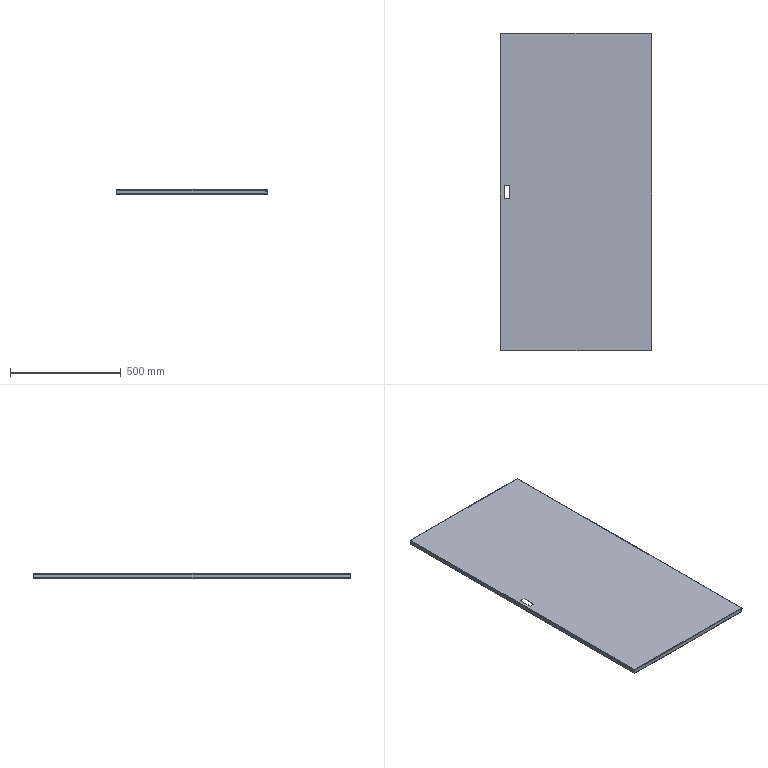Part | SolidWorks | features DelFace 3, BaseBody 1, FlatPattern 1, FlattenBends 1, ProcessBends 1, SheetMetal 1 | 1 solid | 102 faces | box 687 x 1437 x 21 mm | volume 1650433 mm3 | plane 82 | cylinder 20 | commonest cylinder face diameters 0.6 x8 3.6 x8 5.2 x4